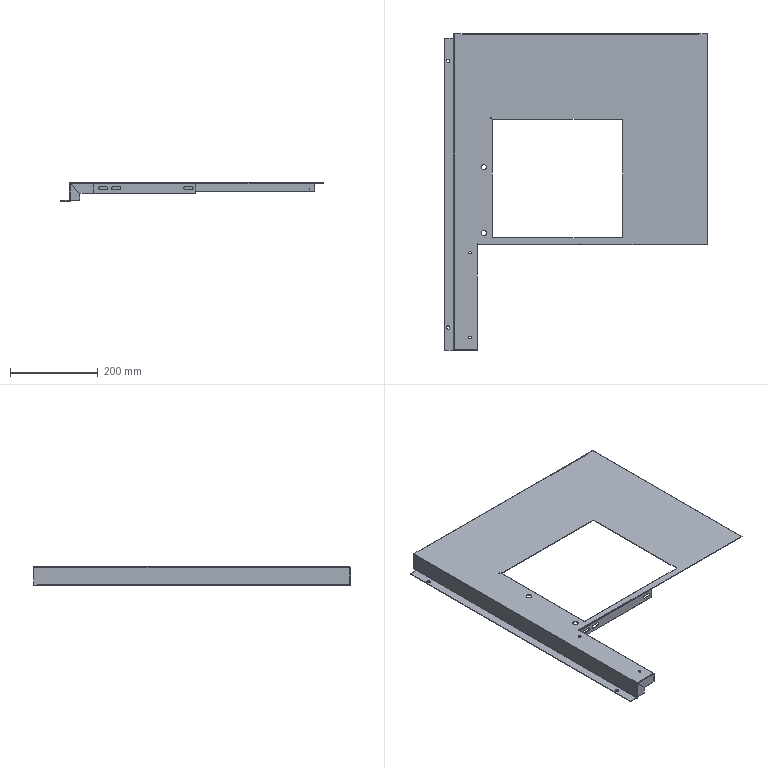Part | SolidWorks | features ICE 8, EdgeFlange 5, LPattern 4, Cut 1, FlatPattern 1, SMBaseFlange 1, SheetMetal 1 | 1 solid | 115 faces | box 600 x 723 x 41.7 mm | volume 406324 mm3 | plane 73 | cylinder 40 | spline 2 | commonest cylinder face diameters 6 x8 0.4 x6 2 x6 3.4 x6 7 x6 7.513 x4